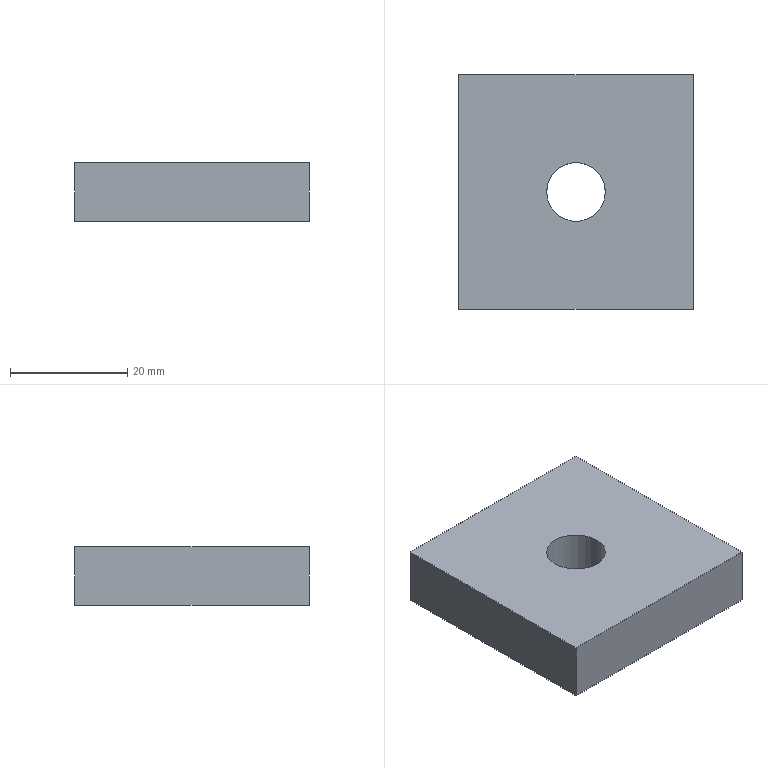Part | SolidWorks | features Extrusion 1 | 1 solid | 8 faces | box 40 x 40 x 10 mm | volume 15215 mm3 | plane 6 | cylinder 2 | commonest cylinder face diameters 10 x2
STEP:
#1=CARTESIAN_POINT('',(15.,20.,10.));
#2=VERTEX_POINT('',#1);
#3=CARTESIAN_POINT('',(25.,20.,10.));
#4=VERTEX_POINT('',#3);
#5=CARTESIAN_POINT('',(20.,20.,10.));
#6=DIRECTION('',(0.,0.,1.));
#7=DIRECTION('',(1.,0.,0.));
#8=AXIS2_PLACEMENT_3D('',#5,#6,#7);
#9=CIRCLE('',#8,5.);
#10=EDGE_CURVE('',#2,#4,#9,.T.);
#11=ORIENTED_EDGE('',*,*,#10,.T.);
#12=CARTESIAN_POINT('',(25.,20.,0.));
#13=VERTEX_POINT('',#12);
#14=CARTESIAN_POINT('',(25.,20.,10.));
#15=DIRECTION('',(0.,0.,-1.));
#16=VECTOR('',#15,1000.);
#17=LINE('',#14,#16);
#18=EDGE_CURVE('',#4,#13,#17,.T.);
#19=ORIENTED_EDGE('',*,*,#18,.T.);
#20=CARTESIAN_POINT('',(15.,20.,0.));
#21=VERTEX_POINT('',#20);
#22=CARTESIAN_POINT('',(20.,20.,0.));
#23=DIRECTION('',(0.,0.,1.));
#24=DIRECTION('',(1.,0.,0.));
#25=AXIS2_PLACEMENT_3D('',#22,#23,#24);
#26=CIRCLE('',#25,5.);
#27=EDGE_CURVE('',#21,#13,#26,.T.);
#28=ORIENTED_EDGE('',*,*,#27,.F.);
#29=CARTESIAN_POINT('',(15.,20.,10.));
#30=DIRECTION('',(0.,0.,-1.));
#31=VECTOR('',#30,1000.);
#32=LINE('',#29,#31);
#33=EDGE_CURVE('',#2,#21,#32,.T.);
#34=ORIENTED_EDGE('',*,*,#33,.F.);
#35=EDGE_LOOP('',(#11,#19,#28,#34));
#36=FACE_OUTER_BOUND('',#35,.T.);
#37=CARTESIAN_POINT('',(20.,20.,10.));
#38=DIRECTION('',(0.,0.,-1.));
#39=DIRECTION('',(-1.,0.,0.));
#40=AXIS2_PLACEMENT_3D('',#37,#38,#39);
#41=CYLINDRICAL_SURFACE('',#40,5.);
#42=ADVANCED_FACE('',(#36),#41,.F.);
#43=CARTESIAN_POINT('',(0.,40.,10.));
#44=VERTEX_POINT('',#43);
#45=CARTESIAN_POINT('',(0.,0.,10.));
#46=VERTEX_POINT('',#45);
#47=CARTESIAN_POINT('',(0.,0.,10.));
#48=DIRECTION('',(0.,-1.,0.));
#49=VECTOR('',#48,1000.);
#50=LINE('',#47,#49);
#51=EDGE_CURVE('',#44,#46,#50,.T.);
#52=ORIENTED_EDGE('',*,*,#51,.T.);
#53=CARTESIAN_POINT('',(40.,0.,10.));
#54=VERTEX_POINT('',#53);
#55=CARTESIAN_POINT('',(0.,0.,10.));
#56=DIRECTION('',(1.,0.,0.));
#57=VECTOR('',#56,1000.);
#58=LINE('',#55,#57);
#59=EDGE_CURVE('',#46,#54,#58,.T.);
#60=ORIENTED_EDGE('',*,*,#59,.T.);
#61=CARTESIAN_POINT('',(40.,40.,10.));
#62=VERTEX_POINT('',#61);
#63=CARTESIAN_POINT('',(40.,0.,10.));
#64=DIRECTION('',(0.,1.,0.));
#65=VECTOR('',#64,1000.);
#66=LINE('',#63,#65);
#67=EDGE_CURVE('',#54,#62,#66,.T.);
#68=ORIENTED_EDGE('',*,*,#67,.T.);
#69=CARTESIAN_POINT('',(0.,40.,10.));
#70=DIRECTION('',(-1.,0.,0.));
#71=VECTOR('',#70,1000.);
#72=LINE('',#69,#71);
#73=EDGE_CURVE('',#62,#44,#72,.T.);
#74=ORIENTED_EDGE('',*,*,#73,.T.);
#75=EDGE_LOOP('',(#52,#60,#68,#74));
#76=FACE_OUTER_BOUND('',#75,.T.);
#77=ORIENTED_EDGE('',*,*,#10,.F.);
#78=CARTESIAN_POINT('',(20.,20.,10.));
#79=DIRECTION('',(0.,0.,1.));
#80=DIRECTION('',(1.,0.,0.));
#81=AXIS2_PLACEMENT_3D('',#78,#79,#80);
#82=CIRCLE('',#81,5.);
#83=EDGE_CURVE('',#4,#2,#82,.T.);
#84=ORIENTED_EDGE('',*,*,#83,.F.);
#85=EDGE_LOOP('',(#77,#84));
#86=FACE_BOUND('',#85,.T.);
#87=CARTESIAN_POINT('',(0.,0.,10.));
#88=DIRECTION('',(0.,0.,-1.));
#89=DIRECTION('',(-1.,0.,0.));
#90=AXIS2_PLACEMENT_3D('',#87,#88,#89);
#91=PLANE('',#90);
#92=ADVANCED_FACE('',(#76,#86),#91,.F.);
#93=CARTESIAN_POINT('',(0.,40.,0.));
#94=VERTEX_POINT('',#93);
#95=CARTESIAN_POINT('',(0.,0.,0.));
#96=VERTEX_POINT('',#95);
#97=CARTESIAN_POINT('',(0.,0.,0.));
#98=DIRECTION('',(0.,-1.,0.));
#99=VECTOR('',#98,1000.);
#100=LINE('',#97,#99);
#101=EDGE_CURVE('',#94,#96,#100,.T.);
#102=ORIENTED_EDGE('',*,*,#101,.F.);
#103=CARTESIAN_POINT('',(40.,40.,0.));
#104=VERTEX_POINT('',#103);
#105=CARTESIAN_POINT('',(0.,40.,0.));
#106=DIRECTION('',(-1.,0.,0.));
#107=VECTOR('',#106,1000.);
#108=LINE('',#105,#107);
#109=EDGE_CURVE('',#104,#94,#108,.T.);
#110=ORIENTED_EDGE('',*,*,#109,.F.);
#111=CARTESIAN_POINT('',(40.,0.,0.));
#112=VERTEX_POINT('',#111);
#113=CARTESIAN_POINT('',(40.,0.,0.));
#114=DIRECTION('',(0.,1.,0.));
#115=VECTOR('',#114,1000.);
#116=LINE('',#113,#115);
#117=EDGE_CURVE('',#112,#104,#116,.T.);
#118=ORIENTED_EDGE('',*,*,#117,.F.);
#119=CARTESIAN_POINT('',(0.,0.,0.));
#120=DIRECTION('',(1.,0.,0.));
#121=VECTOR('',#120,1000.);
#122=LINE('',#119,#121);
#123=EDGE_CURVE('',#96,#112,#122,.T.);
#124=ORIENTED_EDGE('',*,*,#123,.F.);
#125=EDGE_LOOP('',(#102,#110,#118,#124));
#126=FACE_OUTER_BOUND('',#125,.T.);
#127=ORIENTED_EDGE('',*,*,#27,.T.);
#128=CARTESIAN_POINT('',(20.,20.,0.));
#129=DIRECTION('',(0.,0.,1.));
#130=DIRECTION('',(1.,0.,0.));
#131=AXIS2_PLACEMENT_3D('',#128,#129,#130);
#132=CIRCLE('',#131,5.);
#133=EDGE_CURVE('',#13,#21,#132,.T.);
#134=ORIENTED_EDGE('',*,*,#133,.T.);
#135=EDGE_LOOP('',(#127,#134));
#136=FACE_BOUND('',#135,.T.);
#137=CARTESIAN_POINT('',(0.,0.,0.));
#138=DIRECTION('',(0.,0.,-1.));
#139=DIRECTION('',(-1.,0.,0.));
#140=AXIS2_PLACEMENT_3D('',#137,#138,#139);
#141=PLANE('',#140);
#142=ADVANCED_FACE('',(#126,#136),#141,.T.);
#143=ORIENTED_EDGE('',*,*,#101,.T.);
#144=CARTESIAN_POINT('',(0.,0.,10.));
#145=DIRECTION('',(0.,0.,-1.));
#146=VECTOR('',#145,1000.);
#147=LINE('',#144,#146);
#148=EDGE_CURVE('',#46,#96,#147,.T.);
#149=ORIENTED_EDGE('',*,*,#148,.F.);
#150=ORIENTED_EDGE('',*,*,#51,.F.);
#151=CARTESIAN_POINT('',(0.,40.,10.));
#152=DIRECTION('',(0.,0.,-1.));
#153=VECTOR('',#152,1000.);
#154=LINE('',#151,#153);
#155=EDGE_CURVE('',#44,#94,#154,.T.);
#156=ORIENTED_EDGE('',*,*,#155,.T.);
#157=EDGE_LOOP('',(#143,#149,#150,#156));
#158=FACE_OUTER_BOUND('',#157,.T.);
#159=CARTESIAN_POINT('',(0.,0.,10.));
#160=DIRECTION('',(1.,0.,0.));
#161=DIRECTION('',(0.,0.,-1.));
#162=AXIS2_PLACEMENT_3D('',#159,#160,#161);
#163=PLANE('',#162);
#164=ADVANCED_FACE('',(#158),#163,.F.);
#165=ORIENTED_EDGE('',*,*,#123,.T.);
#166=CARTESIAN_POINT('',(40.,0.,10.));
#167=DIRECTION('',(0.,0.,-1.));
#168=VECTOR('',#167,1000.);
#169=LINE('',#166,#168);
#170=EDGE_CURVE('',#54,#112,#169,.T.);
#171=ORIENTED_EDGE('',*,*,#170,.F.);
#172=ORIENTED_EDGE('',*,*,#59,.F.);
#173=ORIENTED_EDGE('',*,*,#148,.T.);
#174=EDGE_LOOP('',(#165,#171,#172,#173));
#175=FACE_OUTER_BOUND('',#174,.T.);
#176=CARTESIAN_POINT('',(0.,0.,10.));
#177=DIRECTION('',(0.,1.,0.));
#178=DIRECTION('',(0.,0.,1.));
#179=AXIS2_PLACEMENT_3D('',#176,#177,#178);
#180=PLANE('',#179);
#181=ADVANCED_FACE('',(#175),#180,.F.);
#182=ORIENTED_EDGE('',*,*,#117,.T.);
#183=CARTESIAN_POINT('',(40.,40.,10.));
#184=DIRECTION('',(0.,0.,-1.));
#185=VECTOR('',#184,1000.);
#186=LINE('',#183,#185);
#187=EDGE_CURVE('',#62,#104,#186,.T.);
#188=ORIENTED_EDGE('',*,*,#187,.F.);
#189=ORIENTED_EDGE('',*,*,#67,.F.);
#190=ORIENTED_EDGE('',*,*,#170,.T.);
#191=EDGE_LOOP('',(#182,#188,#189,#190));
#192=FACE_OUTER_BOUND('',#191,.T.);
#193=CARTESIAN_POINT('',(40.,0.,10.));
#194=DIRECTION('',(-1.,0.,0.));
#195=DIRECTION('',(0.,0.,1.));
#196=AXIS2_PLACEMENT_3D('',#193,#194,#195);
#197=PLANE('',#196);
#198=ADVANCED_FACE('',(#192),#197,.F.);
#199=ORIENTED_EDGE('',*,*,#109,.T.);
#200=ORIENTED_EDGE('',*,*,#155,.F.);
#201=ORIENTED_EDGE('',*,*,#73,.F.);
#202=ORIENTED_EDGE('',*,*,#187,.T.);
#203=EDGE_LOOP('',(#199,#200,#201,#202));
#204=FACE_OUTER_BOUND('',#203,.T.);
#205=CARTESIAN_POINT('',(0.,40.,10.));
#206=DIRECTION('',(0.,-1.,0.));
#207=DIRECTION('',(0.,0.,-1.));
#208=AXIS2_PLACEMENT_3D('',#205,#206,#207);
#209=PLANE('',#208);
#210=ADVANCED_FACE('',(#204),#209,.F.);
#211=ORIENTED_EDGE('',*,*,#18,.F.);
#212=ORIENTED_EDGE('',*,*,#83,.T.);
#213=ORIENTED_EDGE('',*,*,#33,.T.);
#214=ORIENTED_EDGE('',*,*,#133,.F.);
#215=EDGE_LOOP('',(#211,#212,#213,#214));
#216=FACE_OUTER_BOUND('',#215,.T.);
#217=CARTESIAN_POINT('',(20.,20.,10.));
#218=DIRECTION('',(0.,0.,-1.));
#219=DIRECTION('',(-1.,0.,0.));
#220=AXIS2_PLACEMENT_3D('',#217,#218,#219);
#221=CYLINDRICAL_SURFACE('',#220,5.);
#222=ADVANCED_FACE('',(#216),#221,.F.);
#223=CLOSED_SHELL('',(#42,#92,#142,#164,#181,#198,#210,#222));
#224=MANIFOLD_SOLID_BREP('',#223);
#225=CARTESIAN_POINT('',(0.,0.,0.));
#226=DIRECTION('',(0.,0.,1.));
#227=DIRECTION('',(1.,0.,0.));
#228=AXIS2_PLACEMENT_3D('',#225,#226,#227);
#229=(LENGTH_UNIT()NAMED_UNIT(*)SI_UNIT(.MILLI.,.METRE.));
#230=UNCERTAINTY_MEASURE_WITH_UNIT(LENGTH_MEASURE(0.00001),#229,'','');
#231=(NAMED_UNIT(*)PLANE_ANGLE_UNIT()SI_UNIT($,.RADIAN.));
#232=(NAMED_UNIT(*)SI_UNIT($,.STERADIAN.)SOLID_ANGLE_UNIT());
#233=(GEOMETRIC_REPRESENTATION_CONTEXT(3)GLOBAL_UNCERTAINTY_ASSIGNED_CONTEXT((#230))GLOBAL_UNIT_ASSIGNED_CONTEXT((#229,#231,#232))REPRESENTATION_CONTEXT('',''));
#234=ADVANCED_BREP_SHAPE_REPRESENTATION('',(#224,#228),#233);